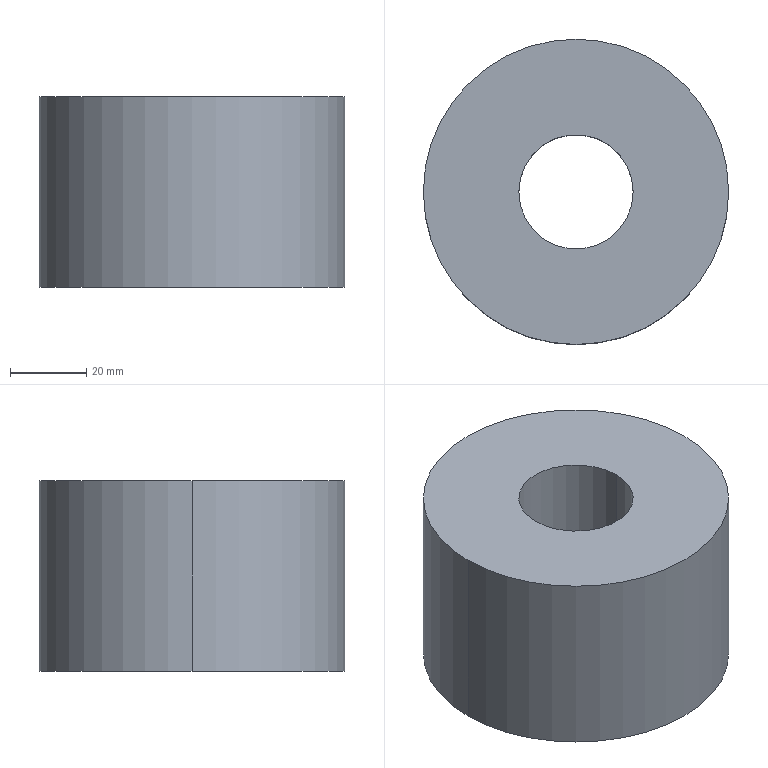Part | SolidWorks | features Extrusion 1 | 1 solid | 6 faces | box 80 x 80 x 50 mm | volume 215984 mm3 | cylinder 4 | plane 2 | commonest cylinder face diameters 30 x2 80 x2
STEP:
#1=CARTESIAN_POINT('',(-15.,0.,50.));
#2=VERTEX_POINT('',#1);
#3=CARTESIAN_POINT('',(15.,0.,50.));
#4=VERTEX_POINT('',#3);
#5=CARTESIAN_POINT('',(0.,0.,50.));
#6=DIRECTION('',(0.,0.,1.));
#7=DIRECTION('',(1.,0.,0.));
#8=AXIS2_PLACEMENT_3D('',#5,#6,#7);
#9=CIRCLE('',#8,15.);
#10=EDGE_CURVE('',#2,#4,#9,.T.);
#11=ORIENTED_EDGE('',*,*,#10,.T.);
#12=CARTESIAN_POINT('',(15.,0.,0.));
#13=VERTEX_POINT('',#12);
#14=CARTESIAN_POINT('',(15.,0.,50.));
#15=DIRECTION('',(0.,0.,-1.));
#16=VECTOR('',#15,1000.);
#17=LINE('',#14,#16);
#18=EDGE_CURVE('',#4,#13,#17,.T.);
#19=ORIENTED_EDGE('',*,*,#18,.T.);
#20=CARTESIAN_POINT('',(-15.,0.,0.));
#21=VERTEX_POINT('',#20);
#22=CARTESIAN_POINT('',(0.,0.,0.));
#23=DIRECTION('',(0.,0.,1.));
#24=DIRECTION('',(1.,0.,0.));
#25=AXIS2_PLACEMENT_3D('',#22,#23,#24);
#26=CIRCLE('',#25,15.);
#27=EDGE_CURVE('',#21,#13,#26,.T.);
#28=ORIENTED_EDGE('',*,*,#27,.F.);
#29=CARTESIAN_POINT('',(-15.,0.,50.));
#30=DIRECTION('',(0.,0.,-1.));
#31=VECTOR('',#30,1000.);
#32=LINE('',#29,#31);
#33=EDGE_CURVE('',#2,#21,#32,.T.);
#34=ORIENTED_EDGE('',*,*,#33,.F.);
#35=EDGE_LOOP('',(#11,#19,#28,#34));
#36=FACE_OUTER_BOUND('',#35,.T.);
#37=CARTESIAN_POINT('',(0.,0.,50.));
#38=DIRECTION('',(0.,0.,-1.));
#39=DIRECTION('',(-1.,0.,0.));
#40=AXIS2_PLACEMENT_3D('',#37,#38,#39);
#41=CYLINDRICAL_SURFACE('',#40,15.);
#42=ADVANCED_FACE('',(#36),#41,.F.);
#43=CARTESIAN_POINT('',(40.,0.,50.));
#44=VERTEX_POINT('',#43);
#45=CARTESIAN_POINT('',(-40.,0.,50.));
#46=VERTEX_POINT('',#45);
#47=CARTESIAN_POINT('',(0.,0.,50.));
#48=DIRECTION('',(0.,0.,1.));
#49=DIRECTION('',(1.,0.,0.));
#50=AXIS2_PLACEMENT_3D('',#47,#48,#49);
#51=CIRCLE('',#50,40.);
#52=EDGE_CURVE('',#44,#46,#51,.T.);
#53=ORIENTED_EDGE('',*,*,#52,.F.);
#54=CARTESIAN_POINT('',(40.,0.,0.));
#55=VERTEX_POINT('',#54);
#56=CARTESIAN_POINT('',(40.,0.,50.));
#57=DIRECTION('',(0.,0.,-1.));
#58=VECTOR('',#57,1000.);
#59=LINE('',#56,#58);
#60=EDGE_CURVE('',#44,#55,#59,.T.);
#61=ORIENTED_EDGE('',*,*,#60,.T.);
#62=CARTESIAN_POINT('',(-40.,0.,0.));
#63=VERTEX_POINT('',#62);
#64=CARTESIAN_POINT('',(0.,0.,0.));
#65=DIRECTION('',(0.,0.,1.));
#66=DIRECTION('',(1.,0.,0.));
#67=AXIS2_PLACEMENT_3D('',#64,#65,#66);
#68=CIRCLE('',#67,40.);
#69=EDGE_CURVE('',#55,#63,#68,.T.);
#70=ORIENTED_EDGE('',*,*,#69,.T.);
#71=CARTESIAN_POINT('',(-40.,0.,50.));
#72=DIRECTION('',(0.,0.,-1.));
#73=VECTOR('',#72,1000.);
#74=LINE('',#71,#73);
#75=EDGE_CURVE('',#46,#63,#74,.T.);
#76=ORIENTED_EDGE('',*,*,#75,.F.);
#77=EDGE_LOOP('',(#53,#61,#70,#76));
#78=FACE_OUTER_BOUND('',#77,.T.);
#79=CARTESIAN_POINT('',(0.,0.,50.));
#80=DIRECTION('',(0.,0.,-1.));
#81=DIRECTION('',(-1.,0.,0.));
#82=AXIS2_PLACEMENT_3D('',#79,#80,#81);
#83=CYLINDRICAL_SURFACE('',#82,40.);
#84=ADVANCED_FACE('',(#78),#83,.T.);
#85=CARTESIAN_POINT('',(0.,0.,50.));
#86=DIRECTION('',(0.,0.,1.));
#87=DIRECTION('',(1.,0.,0.));
#88=AXIS2_PLACEMENT_3D('',#85,#86,#87);
#89=CIRCLE('',#88,40.);
#90=EDGE_CURVE('',#46,#44,#89,.T.);
#91=ORIENTED_EDGE('',*,*,#90,.T.);
#92=ORIENTED_EDGE('',*,*,#52,.T.);
#93=EDGE_LOOP('',(#91,#92));
#94=FACE_OUTER_BOUND('',#93,.T.);
#95=ORIENTED_EDGE('',*,*,#10,.F.);
#96=CARTESIAN_POINT('',(0.,0.,50.));
#97=DIRECTION('',(0.,0.,1.));
#98=DIRECTION('',(1.,0.,0.));
#99=AXIS2_PLACEMENT_3D('',#96,#97,#98);
#100=CIRCLE('',#99,15.);
#101=EDGE_CURVE('',#4,#2,#100,.T.);
#102=ORIENTED_EDGE('',*,*,#101,.F.);
#103=EDGE_LOOP('',(#95,#102));
#104=FACE_BOUND('',#103,.T.);
#105=CARTESIAN_POINT('',(0.,0.,50.));
#106=DIRECTION('',(0.,0.,1.));
#107=DIRECTION('',(1.,0.,0.));
#108=AXIS2_PLACEMENT_3D('',#105,#106,#107);
#109=PLANE('',#108);
#110=ADVANCED_FACE('',(#94,#104),#109,.T.);
#111=CARTESIAN_POINT('',(0.,0.,0.));
#112=DIRECTION('',(0.,0.,1.));
#113=DIRECTION('',(1.,0.,0.));
#114=AXIS2_PLACEMENT_3D('',#111,#112,#113);
#115=CIRCLE('',#114,40.);
#116=EDGE_CURVE('',#63,#55,#115,.T.);
#117=ORIENTED_EDGE('',*,*,#116,.F.);
#118=ORIENTED_EDGE('',*,*,#69,.F.);
#119=EDGE_LOOP('',(#117,#118));
#120=FACE_OUTER_BOUND('',#119,.T.);
#121=ORIENTED_EDGE('',*,*,#27,.T.);
#122=CARTESIAN_POINT('',(0.,0.,0.));
#123=DIRECTION('',(0.,0.,1.));
#124=DIRECTION('',(1.,0.,0.));
#125=AXIS2_PLACEMENT_3D('',#122,#123,#124);
#126=CIRCLE('',#125,15.);
#127=EDGE_CURVE('',#13,#21,#126,.T.);
#128=ORIENTED_EDGE('',*,*,#127,.T.);
#129=EDGE_LOOP('',(#121,#128));
#130=FACE_BOUND('',#129,.T.);
#131=CARTESIAN_POINT('',(0.,0.,0.));
#132=DIRECTION('',(0.,0.,1.));
#133=DIRECTION('',(1.,0.,0.));
#134=AXIS2_PLACEMENT_3D('',#131,#132,#133);
#135=PLANE('',#134);
#136=ADVANCED_FACE('',(#120,#130),#135,.F.);
#137=ORIENTED_EDGE('',*,*,#60,.F.);
#138=ORIENTED_EDGE('',*,*,#90,.F.);
#139=ORIENTED_EDGE('',*,*,#75,.T.);
#140=ORIENTED_EDGE('',*,*,#116,.T.);
#141=EDGE_LOOP('',(#137,#138,#139,#140));
#142=FACE_OUTER_BOUND('',#141,.T.);
#143=CARTESIAN_POINT('',(0.,0.,50.));
#144=DIRECTION('',(0.,0.,-1.));
#145=DIRECTION('',(-1.,0.,0.));
#146=AXIS2_PLACEMENT_3D('',#143,#144,#145);
#147=CYLINDRICAL_SURFACE('',#146,40.);
#148=ADVANCED_FACE('',(#142),#147,.T.);
#149=ORIENTED_EDGE('',*,*,#18,.F.);
#150=ORIENTED_EDGE('',*,*,#101,.T.);
#151=ORIENTED_EDGE('',*,*,#33,.T.);
#152=ORIENTED_EDGE('',*,*,#127,.F.);
#153=EDGE_LOOP('',(#149,#150,#151,#152));
#154=FACE_OUTER_BOUND('',#153,.T.);
#155=CARTESIAN_POINT('',(0.,0.,50.));
#156=DIRECTION('',(0.,0.,-1.));
#157=DIRECTION('',(-1.,0.,0.));
#158=AXIS2_PLACEMENT_3D('',#155,#156,#157);
#159=CYLINDRICAL_SURFACE('',#158,15.);
#160=ADVANCED_FACE('',(#154),#159,.F.);
#161=CLOSED_SHELL('',(#42,#84,#110,#136,#148,#160));
#162=MANIFOLD_SOLID_BREP('',#161);
#163=CARTESIAN_POINT('',(0.,0.,0.));
#164=DIRECTION('',(0.,0.,1.));
#165=DIRECTION('',(1.,0.,0.));
#166=AXIS2_PLACEMENT_3D('',#163,#164,#165);
#167=(LENGTH_UNIT()NAMED_UNIT(*)SI_UNIT(.MILLI.,.METRE.));
#168=UNCERTAINTY_MEASURE_WITH_UNIT(LENGTH_MEASURE(0.00001),#167,'','');
#169=(NAMED_UNIT(*)PLANE_ANGLE_UNIT()SI_UNIT($,.RADIAN.));
#170=(NAMED_UNIT(*)SI_UNIT($,.STERADIAN.)SOLID_ANGLE_UNIT());
#171=(GEOMETRIC_REPRESENTATION_CONTEXT(3)GLOBAL_UNCERTAINTY_ASSIGNED_CONTEXT((#168))GLOBAL_UNIT_ASSIGNED_CONTEXT((#167,#169,#170))REPRESENTATION_CONTEXT('',''));
#172=ADVANCED_BREP_SHAPE_REPRESENTATION('',(#162,#166),#171);